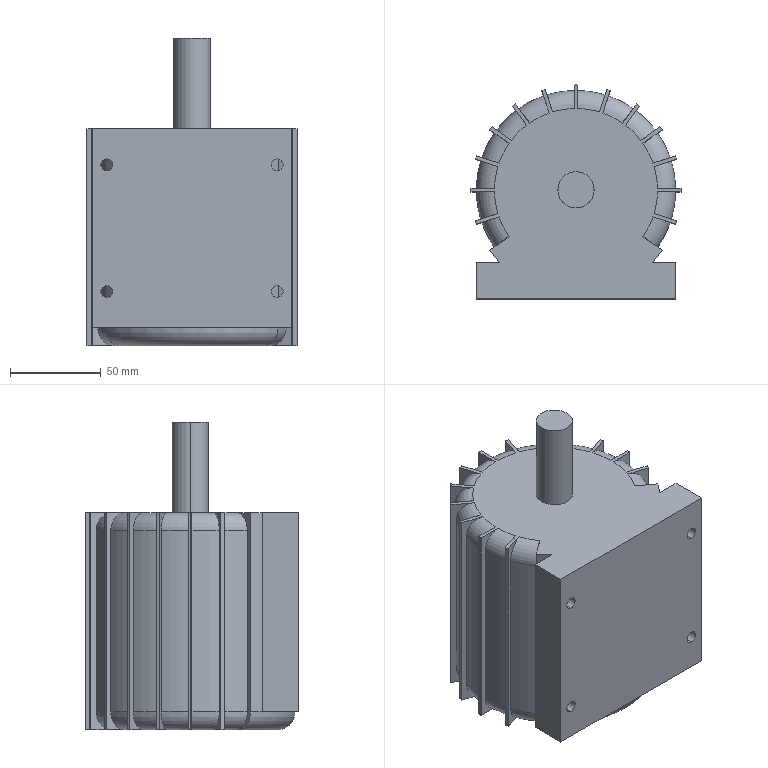Part | NX | 1 solid | 106 faces | box 116 x 118 x 170 mm | volume 1317938 mm3 | cylinder 40 | plane 37 | torus 29 | commonest cylinder face diameters 116 x16 110 x14 6.561 x8 20 x2